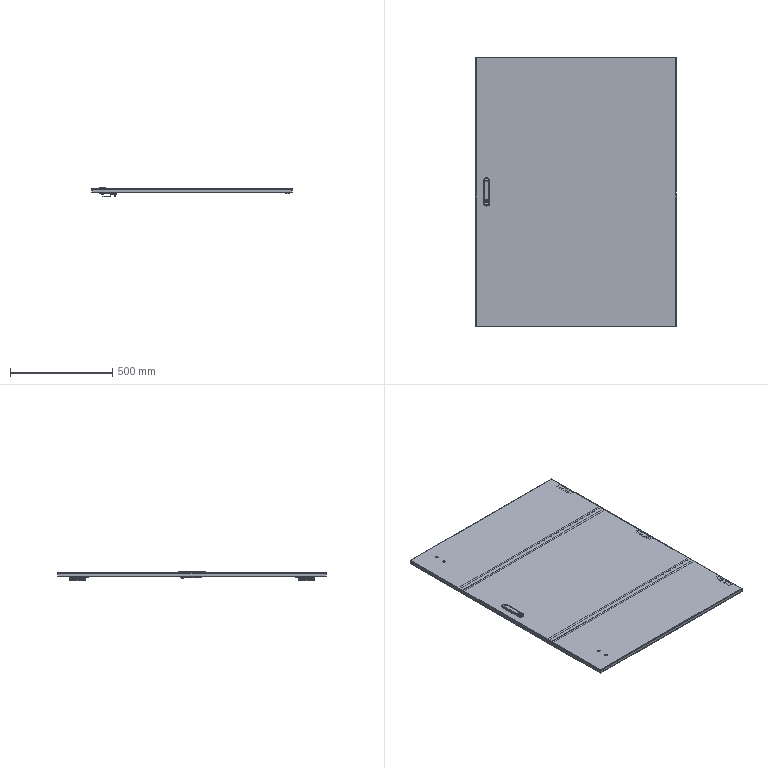Part | NX | features BREP 8 | 18 solids | 883 faces | box 982 x 1320 x 48.621 mm | volume 3205560 mm3 | plane 471 | cylinder 317 | cone 61 | torus 18 | spline 16 | commonest cylinder face diameters 7 x72 12 x36 6 x30 4 x29 10 x22 8 x21